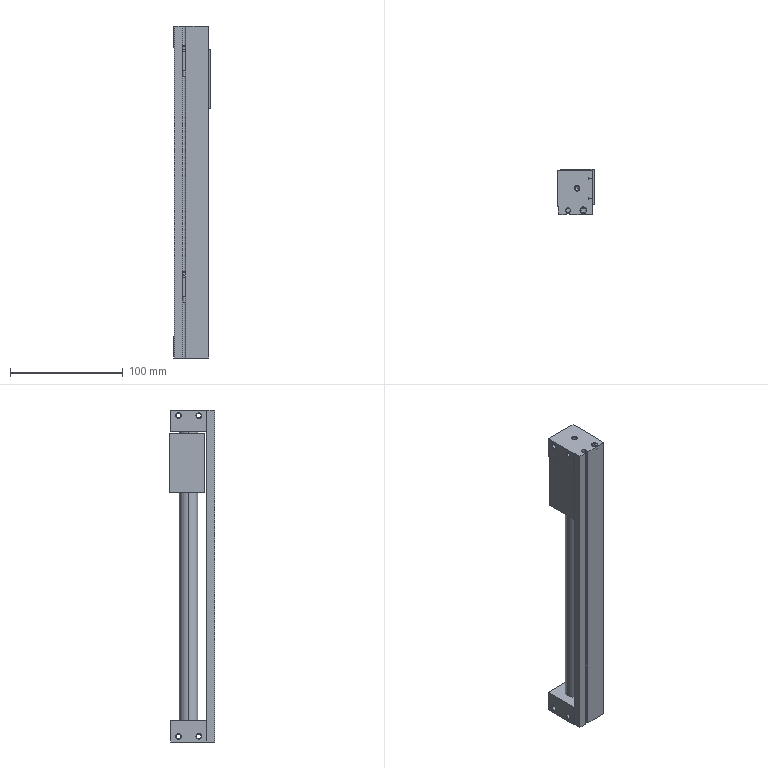Part | STEP file | Magnetically coupled rodless cylinder CY3R15-200 | 4 solids | 205 faces | box 32 x 40 x 294 mm | volume 185652 mm3 | plane 80 | cylinder 77 | cone 48 | commonest cylinder face diameters 3.242 x16 4.134 x12 4.3 x8 8 x8 4 x6 2.5 x4